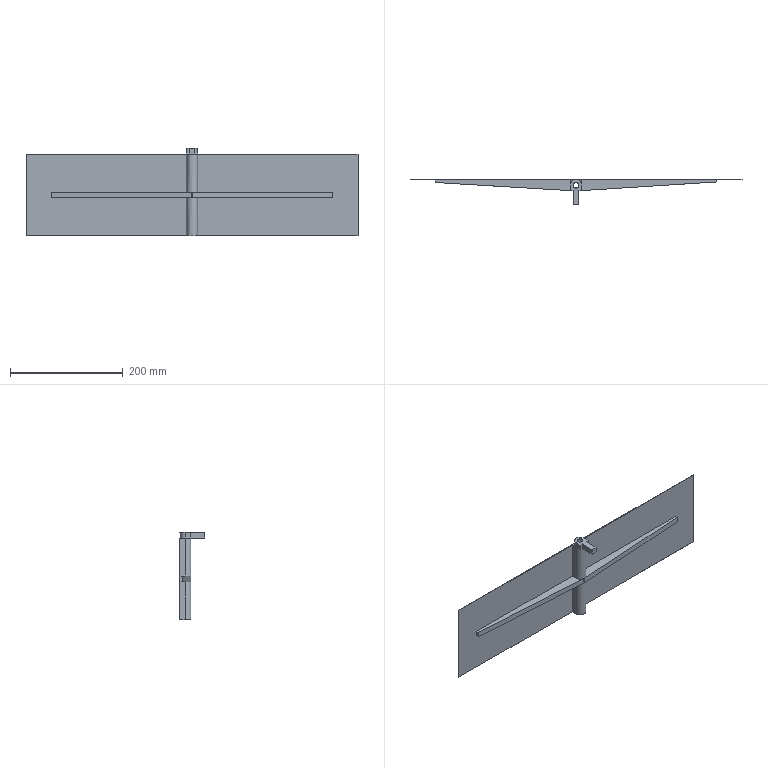Part | SolidWorks | features ICE 3, Extrusion 1 | 1 solid | 32 faces | box 590 x 46 x 155 mm | volume 188951 mm3 | plane 28 | cylinder 4 | commonest cylinder face diameters 10 x2 20 x2
STEP:
#1=CARTESIAN_POINT('',(-5.,0.,82.5));
#2=VERTEX_POINT('',#1);
#3=CARTESIAN_POINT('',(5.,0.,82.5));
#4=VERTEX_POINT('',#3);
#5=CARTESIAN_POINT('',(0.,0.,82.5));
#6=DIRECTION('',(0.,0.,1.));
#7=DIRECTION('',(1.,0.,0.));
#8=AXIS2_PLACEMENT_3D('',#5,#6,#7);
#9=CIRCLE('',#8,5.);
#10=EDGE_CURVE('',#2,#4,#9,.T.);
#11=ORIENTED_EDGE('',*,*,#10,.T.);
#12=CARTESIAN_POINT('',(5.,0.,-72.5));
#13=VERTEX_POINT('',#12);
#14=CARTESIAN_POINT('',(5.,0.,72.5));
#15=DIRECTION('',(0.,0.,-1.));
#16=VECTOR('',#15,1000.);
#17=LINE('',#14,#16);
#18=EDGE_CURVE('',#4,#13,#17,.T.);
#19=ORIENTED_EDGE('',*,*,#18,.T.);
#20=CARTESIAN_POINT('',(-5.,0.,-72.5));
#21=VERTEX_POINT('',#20);
#22=CARTESIAN_POINT('',(0.,0.,-72.5));
#23=DIRECTION('',(0.,0.,1.));
#24=DIRECTION('',(1.,0.,0.));
#25=AXIS2_PLACEMENT_3D('',#22,#23,#24);
#26=CIRCLE('',#25,5.);
#27=EDGE_CURVE('',#21,#13,#26,.T.);
#28=ORIENTED_EDGE('',*,*,#27,.F.);
#29=CARTESIAN_POINT('',(-5.,0.,72.5));
#30=DIRECTION('',(0.,0.,-1.));
#31=VECTOR('',#30,1000.);
#32=LINE('',#29,#31);
#33=EDGE_CURVE('',#2,#21,#32,.T.);
#34=ORIENTED_EDGE('',*,*,#33,.F.);
#35=EDGE_LOOP('',(#11,#19,#28,#34));
#36=FACE_OUTER_BOUND('',#35,.T.);
#37=CARTESIAN_POINT('',(0.,0.,72.5));
#38=DIRECTION('',(0.,0.,-1.));
#39=DIRECTION('',(-1.,0.,0.));
#40=AXIS2_PLACEMENT_3D('',#37,#38,#39);
#41=CYLINDRICAL_SURFACE('',#40,5.);
#42=ADVANCED_FACE('',(#36),#41,.F.);
#43=CARTESIAN_POINT('',(10.,10.,-5.));
#44=VERTEX_POINT('',#43);
#45=CARTESIAN_POINT('',(10.,0.,-5.));
#46=VERTEX_POINT('',#45);
#47=CARTESIAN_POINT('',(10.,0.,-5.));
#48=DIRECTION('',(0.,-1.,0.));
#49=VECTOR('',#48,1000.);
#50=LINE('',#47,#49);
#51=EDGE_CURVE('',#44,#46,#50,.T.);
#52=ORIENTED_EDGE('',*,*,#51,.T.);
#53=CARTESIAN_POINT('',(10.,0.,-72.5));
#54=VERTEX_POINT('',#53);
#55=CARTESIAN_POINT('',(10.,0.,72.5));
#56=DIRECTION('',(0.,0.,-1.));
#57=VECTOR('',#56,1000.);
#58=LINE('',#55,#57);
#59=EDGE_CURVE('',#46,#54,#58,.T.);
#60=ORIENTED_EDGE('',*,*,#59,.T.);
#61=CARTESIAN_POINT('',(10.,10.,-72.5));
#62=VERTEX_POINT('',#61);
#63=CARTESIAN_POINT('',(10.,10.,-72.5));
#64=DIRECTION('',(0.,1.,0.));
#65=VECTOR('',#64,1000.);
#66=LINE('',#63,#65);
#67=EDGE_CURVE('',#54,#62,#66,.T.);
#68=ORIENTED_EDGE('',*,*,#67,.T.);
#69=CARTESIAN_POINT('',(10.,10.,72.5));
#70=DIRECTION('',(0.,0.,-1.));
#71=VECTOR('',#70,1000.);
#72=LINE('',#69,#71);
#73=EDGE_CURVE('',#44,#62,#72,.T.);
#74=ORIENTED_EDGE('',*,*,#73,.F.);
#75=EDGE_LOOP('',(#52,#60,#68,#74));
#76=FACE_OUTER_BOUND('',#75,.T.);
#77=CARTESIAN_POINT('',(10.,10.,72.5));
#78=DIRECTION('',(-1.,0.,0.));
#79=DIRECTION('',(0.,0.,1.));
#80=AXIS2_PLACEMENT_3D('',#77,#78,#79);
#81=PLANE('',#80);
#82=ADVANCED_FACE('',(#76),#81,.F.);
#83=CARTESIAN_POINT('',(-10.,0.,-5.));
#84=VERTEX_POINT('',#83);
#85=CARTESIAN_POINT('',(-10.,10.,-5.));
#86=VERTEX_POINT('',#85);
#87=CARTESIAN_POINT('',(-10.,10.,-5.));
#88=DIRECTION('',(0.,1.,0.));
#89=VECTOR('',#88,1000.);
#90=LINE('',#87,#89);
#91=EDGE_CURVE('',#84,#86,#90,.T.);
#92=ORIENTED_EDGE('',*,*,#91,.T.);
#93=CARTESIAN_POINT('',(-10.,10.,-72.5));
#94=VERTEX_POINT('',#93);
#95=CARTESIAN_POINT('',(-10.,10.,72.5));
#96=DIRECTION('',(0.,0.,-1.));
#97=VECTOR('',#96,1000.);
#98=LINE('',#95,#97);
#99=EDGE_CURVE('',#86,#94,#98,.T.);
#100=ORIENTED_EDGE('',*,*,#99,.T.);
#101=CARTESIAN_POINT('',(-10.,0.,-72.5));
#102=VERTEX_POINT('',#101);
#103=CARTESIAN_POINT('',(-10.,0.,-72.5));
#104=DIRECTION('',(0.,-1.,0.));
#105=VECTOR('',#104,1000.);
#106=LINE('',#103,#105);
#107=EDGE_CURVE('',#94,#102,#106,.T.);
#108=ORIENTED_EDGE('',*,*,#107,.T.);
#109=CARTESIAN_POINT('',(-10.,0.,72.5));
#110=DIRECTION('',(0.,0.,-1.));
#111=VECTOR('',#110,1000.);
#112=LINE('',#109,#111);
#113=EDGE_CURVE('',#84,#102,#112,.T.);
#114=ORIENTED_EDGE('',*,*,#113,.F.);
#115=EDGE_LOOP('',(#92,#100,#108,#114));
#116=FACE_OUTER_BOUND('',#115,.T.);
#117=CARTESIAN_POINT('',(-10.,0.,72.5));
#118=DIRECTION('',(1.,0.,0.));
#119=DIRECTION('',(0.,0.,-1.));
#120=AXIS2_PLACEMENT_3D('',#117,#118,#119);
#121=PLANE('',#120);
#122=ADVANCED_FACE('',(#116),#121,.F.);
#123=CARTESIAN_POINT('',(10.,0.,72.5));
#124=VERTEX_POINT('',#123);
#125=CARTESIAN_POINT('',(-10.,0.,72.5));
#126=VERTEX_POINT('',#125);
#127=CARTESIAN_POINT('',(0.,0.,72.5));
#128=DIRECTION('',(0.,0.,1.));
#129=DIRECTION('',(1.,0.,0.));
#130=AXIS2_PLACEMENT_3D('',#127,#128,#129);
#131=CIRCLE('',#130,10.);
#132=EDGE_CURVE('',#124,#126,#131,.T.);
#133=ORIENTED_EDGE('',*,*,#132,.F.);
#134=CARTESIAN_POINT('',(10.,10.,72.5));
#135=VERTEX_POINT('',#134);
#136=CARTESIAN_POINT('',(10.,10.,72.5));
#137=DIRECTION('',(0.,1.,0.));
#138=VECTOR('',#137,1000.);
#139=LINE('',#136,#138);
#140=EDGE_CURVE('',#124,#135,#139,.T.);
#141=ORIENTED_EDGE('',*,*,#140,.T.);
#142=CARTESIAN_POINT('',(295.,10.,72.5));
#143=VERTEX_POINT('',#142);
#144=CARTESIAN_POINT('',(-295.,10.,72.5));
#145=DIRECTION('',(1.,0.,0.));
#146=VECTOR('',#145,1000.);
#147=LINE('',#144,#146);
#148=EDGE_CURVE('',#135,#143,#147,.T.);
#149=ORIENTED_EDGE('',*,*,#148,.T.);
#150=CARTESIAN_POINT('',(295.,11.,72.5));
#151=VERTEX_POINT('',#150);
#152=CARTESIAN_POINT('',(295.,11.,72.5));
#153=DIRECTION('',(0.,-1.,0.));
#154=VECTOR('',#153,1000.);
#155=LINE('',#152,#154);
#156=EDGE_CURVE('',#151,#143,#155,.T.);
#157=ORIENTED_EDGE('',*,*,#156,.F.);
#158=CARTESIAN_POINT('',(-295.,11.,72.5));
#159=VERTEX_POINT('',#158);
#160=CARTESIAN_POINT('',(-295.,11.,72.5));
#161=DIRECTION('',(1.,0.,0.));
#162=VECTOR('',#161,1000.);
#163=LINE('',#160,#162);
#164=EDGE_CURVE('',#159,#151,#163,.T.);
#165=ORIENTED_EDGE('',*,*,#164,.F.);
#166=CARTESIAN_POINT('',(-295.,10.,72.5));
#167=VERTEX_POINT('',#166);
#168=CARTESIAN_POINT('',(-295.,11.,72.5));
#169=DIRECTION('',(0.,-1.,0.));
#170=VECTOR('',#169,1000.);
#171=LINE('',#168,#170);
#172=EDGE_CURVE('',#159,#167,#171,.T.);
#173=ORIENTED_EDGE('',*,*,#172,.T.);
#174=CARTESIAN_POINT('',(-10.,10.,72.5));
#175=VERTEX_POINT('',#174);
#176=CARTESIAN_POINT('',(-295.,10.,72.5));
#177=DIRECTION('',(1.,0.,0.));
#178=VECTOR('',#177,1000.);
#179=LINE('',#176,#178);
#180=EDGE_CURVE('',#167,#175,#179,.T.);
#181=ORIENTED_EDGE('',*,*,#180,.T.);
#182=CARTESIAN_POINT('',(-10.,0.,72.5));
#183=DIRECTION('',(0.,-1.,0.));
#184=VECTOR('',#183,1000.);
#185=LINE('',#182,#184);
#186=EDGE_CURVE('',#175,#126,#185,.T.);
#187=ORIENTED_EDGE('',*,*,#186,.T.);
#188=EDGE_LOOP('',(#133,#141,#149,#157,#165,#173,#181,#187));
#189=FACE_OUTER_BOUND('',#188,.T.);
#190=CARTESIAN_POINT('',(0.,0.,72.5));
#191=DIRECTION('',(0.,0.,1.));
#192=DIRECTION('',(1.,0.,0.));
#193=AXIS2_PLACEMENT_3D('',#190,#191,#192);
#194=PLANE('',#193);
#195=ADVANCED_FACE('',(#189),#194,.T.);
#196=CARTESIAN_POINT('',(0.,0.,-72.5));
#197=DIRECTION('',(0.,0.,1.));
#198=DIRECTION('',(1.,0.,0.));
#199=AXIS2_PLACEMENT_3D('',#196,#197,#198);
#200=CIRCLE('',#199,10.);
#201=EDGE_CURVE('',#102,#54,#200,.T.);
#202=ORIENTED_EDGE('',*,*,#201,.F.);
#203=ORIENTED_EDGE('',*,*,#107,.F.);
#204=CARTESIAN_POINT('',(-295.,10.,-72.5));
#205=VERTEX_POINT('',#204);
#206=CARTESIAN_POINT('',(-295.,10.,-72.5));
#207=DIRECTION('',(-1.,0.,0.));
#208=VECTOR('',#207,1000.);
#209=LINE('',#206,#208);
#210=EDGE_CURVE('',#94,#205,#209,.T.);
#211=ORIENTED_EDGE('',*,*,#210,.T.);
#212=CARTESIAN_POINT('',(-295.,11.,-72.5));
#213=VERTEX_POINT('',#212);
#214=CARTESIAN_POINT('',(-295.,11.,-72.5));
#215=DIRECTION('',(0.,-1.,0.));
#216=VECTOR('',#215,1000.);
#217=LINE('',#214,#216);
#218=EDGE_CURVE('',#213,#205,#217,.T.);
#219=ORIENTED_EDGE('',*,*,#218,.F.);
#220=CARTESIAN_POINT('',(295.,11.,-72.5));
#221=VERTEX_POINT('',#220);
#222=CARTESIAN_POINT('',(-295.,11.,-72.5));
#223=DIRECTION('',(-1.,0.,0.));
#224=VECTOR('',#223,1000.);
#225=LINE('',#222,#224);
#226=EDGE_CURVE('',#221,#213,#225,.T.);
#227=ORIENTED_EDGE('',*,*,#226,.F.);
#228=CARTESIAN_POINT('',(295.,10.,-72.5));
#229=VERTEX_POINT('',#228);
#230=CARTESIAN_POINT('',(295.,11.,-72.5));
#231=DIRECTION('',(0.,-1.,0.));
#232=VECTOR('',#231,1000.);
#233=LINE('',#230,#232);
#234=EDGE_CURVE('',#221,#229,#233,.T.);
#235=ORIENTED_EDGE('',*,*,#234,.T.);
#236=CARTESIAN_POINT('',(-295.,10.,-72.5));
#237=DIRECTION('',(-1.,0.,0.));
#238=VECTOR('',#237,1000.);
#239=LINE('',#236,#238);
#240=EDGE_CURVE('',#229,#62,#239,.T.);
#241=ORIENTED_EDGE('',*,*,#240,.T.);
#242=ORIENTED_EDGE('',*,*,#67,.F.);
#243=EDGE_LOOP('',(#202,#203,#211,#219,#227,#235,#241,#242));
#244=FACE_OUTER_BOUND('',#243,.T.);
#245=ORIENTED_EDGE('',*,*,#27,.T.);
#246=CARTESIAN_POINT('',(0.,0.,-72.5));
#247=DIRECTION('',(0.,0.,1.));
#248=DIRECTION('',(1.,0.,0.));
#249=AXIS2_PLACEMENT_3D('',#246,#247,#248);
#250=CIRCLE('',#249,5.);
#251=EDGE_CURVE('',#13,#21,#250,.T.);
#252=ORIENTED_EDGE('',*,*,#251,.T.);
#253=EDGE_LOOP('',(#245,#252));
#254=FACE_BOUND('',#253,.T.);
#255=CARTESIAN_POINT('',(0.,0.,-72.5));
#256=DIRECTION('',(0.,0.,1.));
#257=DIRECTION('',(1.,0.,0.));
#258=AXIS2_PLACEMENT_3D('',#255,#256,#257);
#259=PLANE('',#258);
#260=ADVANCED_FACE('',(#244,#254),#259,.F.);
#261=CARTESIAN_POINT('',(0.6395,-9.98,5.));
#262=VERTEX_POINT('',#261);
#263=CARTESIAN_POINT('',(0.6395,-9.98,-5.));
#264=VERTEX_POINT('',#263);
#265=CARTESIAN_POINT('',(0.6395,-9.98,5.));
#266=DIRECTION('',(0.,0.,-1.));
#267=VECTOR('',#266,1000.);
#268=LINE('',#265,#267);
#269=EDGE_CURVE('',#262,#264,#268,.T.);
#270=ORIENTED_EDGE('',*,*,#269,.F.);
#271=CARTESIAN_POINT('',(10.,0.,5.));
#272=VERTEX_POINT('',#271);
#273=CARTESIAN_POINT('',(0.,0.,5.));
#274=DIRECTION('',(0.,0.,-1.));
#275=DIRECTION('',(1.,0.,0.));
#276=AXIS2_PLACEMENT_3D('',#273,#274,#275);
#277=CIRCLE('',#276,10.);
#278=EDGE_CURVE('',#272,#262,#277,.T.);
#279=ORIENTED_EDGE('',*,*,#278,.F.);
#280=CARTESIAN_POINT('',(10.,0.,72.5));
#281=DIRECTION('',(0.,0.,-1.));
#282=VECTOR('',#281,1000.);
#283=LINE('',#280,#282);
#284=EDGE_CURVE('',#124,#272,#283,.T.);
#285=ORIENTED_EDGE('',*,*,#284,.F.);
#286=CARTESIAN_POINT('',(0.,0.,72.5));
#287=DIRECTION('',(0.,0.,1.));
#288=DIRECTION('',(1.,0.,0.));
#289=AXIS2_PLACEMENT_3D('',#286,#287,#288);
#290=CIRCLE('',#289,10.);
#291=EDGE_CURVE('',#126,#124,#290,.T.);
#292=ORIENTED_EDGE('',*,*,#291,.F.);
#293=CARTESIAN_POINT('',(-10.,0.,5.));
#294=VERTEX_POINT('',#293);
#295=CARTESIAN_POINT('',(-10.,0.,72.5));
#296=DIRECTION('',(0.,0.,-1.));
#297=VECTOR('',#296,1000.);
#298=LINE('',#295,#297);
#299=EDGE_CURVE('',#126,#294,#298,.T.);
#300=ORIENTED_EDGE('',*,*,#299,.T.);
#301=CARTESIAN_POINT('',(-0.5996,-9.982,5.));
#302=VERTEX_POINT('',#301);
#303=CARTESIAN_POINT('',(0.,0.,5.));
#304=DIRECTION('',(0.,0.,-1.));
#305=DIRECTION('',(1.,0.,0.));
#306=AXIS2_PLACEMENT_3D('',#303,#304,#305);
#307=CIRCLE('',#306,10.);
#308=EDGE_CURVE('',#302,#294,#307,.T.);
#309=ORIENTED_EDGE('',*,*,#308,.F.);
#310=CARTESIAN_POINT('',(-0.5996,-9.982,-5.));
#311=VERTEX_POINT('',#310);
#312=CARTESIAN_POINT('',(-0.5996,-9.982,5.));
#313=DIRECTION('',(0.,0.,-1.));
#314=VECTOR('',#313,1000.);
#315=LINE('',#312,#314);
#316=EDGE_CURVE('',#302,#311,#315,.T.);
#317=ORIENTED_EDGE('',*,*,#316,.T.);
#318=CARTESIAN_POINT('',(0.,0.,-5.));
#319=DIRECTION('',(0.,0.,-1.));
#320=DIRECTION('',(1.,0.,0.));
#321=AXIS2_PLACEMENT_3D('',#318,#319,#320);
#322=CIRCLE('',#321,10.);
#323=EDGE_CURVE('',#311,#84,#322,.T.);
#324=ORIENTED_EDGE('',*,*,#323,.T.);
#325=ORIENTED_EDGE('',*,*,#113,.T.);
#326=ORIENTED_EDGE('',*,*,#201,.T.);
#327=ORIENTED_EDGE('',*,*,#59,.F.);
#328=CARTESIAN_POINT('',(0.,0.,-5.));
#329=DIRECTION('',(0.,0.,-1.));
#330=DIRECTION('',(1.,0.,0.));
#331=AXIS2_PLACEMENT_3D('',#328,#329,#330);
#332=CIRCLE('',#331,10.);
#333=EDGE_CURVE('',#46,#264,#332,.T.);
#334=ORIENTED_EDGE('',*,*,#333,.T.);
#335=EDGE_LOOP('',(#270,#279,#285,#292,#300,#309,#317,#324,#325,#326,#327,#334));
#336=FACE_OUTER_BOUND('',#335,.T.);
#337=CARTESIAN_POINT('',(0.,0.,72.5));
#338=DIRECTION('',(0.,0.,-1.));
#339=DIRECTION('',(-1.,0.,0.));
#340=AXIS2_PLACEMENT_3D('',#337,#338,#339);
#341=CYLINDRICAL_SURFACE('',#340,10.);
#342=ADVANCED_FACE('',(#336),#341,.T.);
#343=ORIENTED_EDGE('',*,*,#284,.T.);
#344=CARTESIAN_POINT('',(10.,10.,5.));
#345=VERTEX_POINT('',#344);
#346=CARTESIAN_POINT('',(10.,0.,5.));
#347=DIRECTION('',(0.,-1.,0.));
#348=VECTOR('',#347,1000.);
#349=LINE('',#346,#348);
#350=EDGE_CURVE('',#345,#272,#349,.T.);
#351=ORIENTED_EDGE('',*,*,#350,.F.);
#352=CARTESIAN_POINT('',(10.,10.,72.5));
#353=DIRECTION('',(0.,0.,-1.));
#354=VECTOR('',#353,1000.);
#355=LINE('',#352,#354);
#356=EDGE_CURVE('',#135,#345,#355,.T.);
#357=ORIENTED_EDGE('',*,*,#356,.F.);
#358=ORIENTED_EDGE('',*,*,#140,.F.);
#359=EDGE_LOOP('',(#343,#351,#357,#358));
#360=FACE_OUTER_BOUND('',#359,.T.);
#361=CARTESIAN_POINT('',(10.,10.,72.5));
#362=DIRECTION('',(-1.,0.,0.));
#363=DIRECTION('',(0.,0.,1.));
#364=AXIS2_PLACEMENT_3D('',#361,#362,#363);
#365=PLANE('',#364);
#366=ADVANCED_FACE('',(#360),#365,.F.);
#367=CARTESIAN_POINT('',(-10.,10.,5.));
#368=VERTEX_POINT('',#367);
#369=CARTESIAN_POINT('',(-10.,10.,72.5));
#370=DIRECTION('',(0.,0.,-1.));
#371=VECTOR('',#370,1000.);
#372=LINE('',#369,#371);
#373=EDGE_CURVE('',#175,#368,#372,.T.);
#374=ORIENTED_EDGE('',*,*,#373,.T.);
#375=CARTESIAN_POINT('',(-10.,10.,5.));
#376=DIRECTION('',(0.,1.,0.));
#377=VECTOR('',#376,1000.);
#378=LINE('',#375,#377);
#379=EDGE_CURVE('',#294,#368,#378,.T.);
#380=ORIENTED_EDGE('',*,*,#379,.F.);
#381=ORIENTED_EDGE('',*,*,#299,.F.);
#382=ORIENTED_EDGE('',*,*,#186,.F.);
#383=EDGE_LOOP('',(#374,#380,#381,#382));
#384=FACE_OUTER_BOUND('',#383,.T.);
#385=CARTESIAN_POINT('',(-10.,0.,72.5));
#386=DIRECTION('',(1.,0.,0.));
#387=DIRECTION('',(0.,0.,-1.));
#388=AXIS2_PLACEMENT_3D('',#385,#386,#387);
#389=PLANE('',#388);
#390=ADVANCED_FACE('',(#384),#389,.F.);
#391=ORIENTED_EDGE('',*,*,#18,.F.);
#392=CARTESIAN_POINT('',(0.,0.,82.5));
#393=DIRECTION('',(0.,0.,1.));
#394=DIRECTION('',(1.,0.,0.));
#395=AXIS2_PLACEMENT_3D('',#392,#393,#394);
#396=CIRCLE('',#395,5.);
#397=EDGE_CURVE('',#4,#2,#396,.T.);
#398=ORIENTED_EDGE('',*,*,#397,.T.);
#399=ORIENTED_EDGE('',*,*,#33,.T.);
#400=ORIENTED_EDGE('',*,*,#251,.F.);
#401=EDGE_LOOP('',(#391,#398,#399,#400));
#402=FACE_OUTER_BOUND('',#401,.T.);
#403=CARTESIAN_POINT('',(0.,0.,72.5));
#404=DIRECTION('',(0.,0.,-1.));
#405=DIRECTION('',(-1.,0.,0.));
#406=AXIS2_PLACEMENT_3D('',#403,#404,#405);
#407=CYLINDRICAL_SURFACE('',#406,5.);
#408=ADVANCED_FACE('',(#402),#407,.F.);
#409=CARTESIAN_POINT('',(-250.,10.,-5.));
#410=VERTEX_POINT('',#409);
#411=CARTESIAN_POINT('',(-250.,5.,-5.));
#412=VERTEX_POINT('',#411);
#413=CARTESIAN_POINT('',(-250.,10.,-5.));
#414=DIRECTION('',(0.,-1.,0.));
#415=VECTOR('',#414,1000.);
#416=LINE('',#413,#415);
#417=EDGE_CURVE('',#410,#412,#416,.T.);
#418=ORIENTED_EDGE('',*,*,#417,.T.);
#419=CARTESIAN_POINT('',(-250.,5.,5.));
#420=VERTEX_POINT('',#419);
#421=CARTESIAN_POINT('',(-250.,5.,5.));
#422=DIRECTION('',(0.,0.,-1.));
#423=VECTOR('',#422,1000.);
#424=LINE('',#421,#423);
#425=EDGE_CURVE('',#420,#412,#424,.T.);
#426=ORIENTED_EDGE('',*,*,#425,.F.);
#427=CARTESIAN_POINT('',(-250.,10.,5.));
#428=VERTEX_POINT('',#427);
#429=CARTESIAN_POINT('',(-250.,10.,5.));
#430=DIRECTION('',(0.,-1.,0.));
#431=VECTOR('',#430,1000.);
#432=LINE('',#429,#431);
#433=EDGE_CURVE('',#428,#420,#432,.T.);
#434=ORIENTED_EDGE('',*,*,#433,.F.);
#435=CARTESIAN_POINT('',(-250.,10.,5.));
#436=DIRECTION('',(0.,0.,-1.));
#437=VECTOR('',#436,1000.);
#438=LINE('',#435,#437);
#439=EDGE_CURVE('',#428,#410,#438,.T.);
#440=ORIENTED_EDGE('',*,*,#439,.T.);
#441=EDGE_LOOP('',(#418,#426,#434,#440));
#442=FACE_OUTER_BOUND('',#441,.T.);
#443=CARTESIAN_POINT('',(-250.,10.,5.));
#444=DIRECTION('',(1.,0.,0.));
#445=DIRECTION('',(0.,0.,-1.));
#446=AXIS2_PLACEMENT_3D('',#443,#444,#445);
#447=PLANE('',#446);
#448=ADVANCED_FACE('',(#442),#447,.F.);
#449=CARTESIAN_POINT('',(-250.,5.,-5.));
#450=DIRECTION('',(0.9982,-0.05996,0.));
#451=VECTOR('',#450,1000.);
#452=LINE('',#449,#451);
#453=EDGE_CURVE('',#412,#311,#452,.T.);
#454=ORIENTED_EDGE('',*,*,#453,.T.);
#455=ORIENTED_EDGE('',*,*,#316,.F.);
#456=CARTESIAN_POINT('',(-250.,5.,5.));
#457=DIRECTION('',(0.9982,-0.05996,0.));
#458=VECTOR('',#457,1000.);
#459=LINE('',#456,#458);
#460=EDGE_CURVE('',#420,#302,#459,.T.);
#461=ORIENTED_EDGE('',*,*,#460,.F.);
#462=ORIENTED_EDGE('',*,*,#425,.T.);
#463=EDGE_LOOP('',(#454,#455,#461,#462));
#464=FACE_OUTER_BOUND('',#463,.T.);
#465=CARTESIAN_POINT('',(-250.,5.,5.));
#466=DIRECTION('',(0.05996,0.9982,0.));
#467=DIRECTION('',(-0.9982,0.05996,0.));
#468=AXIS2_PLACEMENT_3D('',#465,#466,#467);
#469=PLANE('',#468);
#470=ADVANCED_FACE('',(#464),#469,.F.);
#471=ORIENTED_EDGE('',*,*,#379,.T.);
#472=CARTESIAN_POINT('',(-10.,10.,5.));
#473=DIRECTION('',(-1.,0.,0.));
#474=VECTOR('',#473,1000.);
#475=LINE('',#472,#474);
#476=EDGE_CURVE('',#368,#428,#475,.T.);
#477=ORIENTED_EDGE('',*,*,#476,.T.);
#478=ORIENTED_EDGE('',*,*,#433,.T.);
#479=ORIENTED_EDGE('',*,*,#460,.T.);
#480=ORIENTED_EDGE('',*,*,#308,.T.);
#481=EDGE_LOOP('',(#471,#477,#478,#479,#480));
#482=FACE_OUTER_BOUND('',#481,.T.);
#483=CARTESIAN_POINT('',(0.,0.,5.));
#484=DIRECTION('',(0.,0.,1.));
#485=DIRECTION('',(1.,0.,0.));
#486=AXIS2_PLACEMENT_3D('',#483,#484,#485);
#487=PLANE('',#486);
#488=ADVANCED_FACE('',(#482),#487,.T.);
#489=ORIENTED_EDGE('',*,*,#91,.F.);
#490=ORIENTED_EDGE('',*,*,#323,.F.);
#491=ORIENTED_EDGE('',*,*,#453,.F.);
#492=ORIENTED_EDGE('',*,*,#417,.F.);
#493=CARTESIAN_POINT('',(-10.,10.,-5.));
#494=DIRECTION('',(-1.,0.,0.));
#495=VECTOR('',#494,1000.);
#496=LINE('',#493,#495);
#497=EDGE_CURVE('',#86,#410,#496,.T.);
#498=ORIENTED_EDGE('',*,*,#497,.F.);
#499=EDGE_LOOP('',(#489,#490,#491,#492,#498));
#500=FACE_OUTER_BOUND('',#499,.T.);
#501=CARTESIAN_POINT('',(0.,0.,-5.));
#502=DIRECTION('',(0.,0.,1.));
#503=DIRECTION('',(1.,0.,0.));
#504=AXIS2_PLACEMENT_3D('',#501,#502,#503);
#505=PLANE('',#504);
#506=ADVANCED_FACE('',(#500),#505,.F.);
#507=ORIENTED_EDGE('',*,*,#356,.T.);
#508=CARTESIAN_POINT('',(249.998,10.,5.));
#509=VERTEX_POINT('',#508);
#510=CARTESIAN_POINT('',(0.,10.,5.));
#511=DIRECTION('',(1.,0.,0.));
#512=VECTOR('',#511,1000.);
#513=LINE('',#510,#512);
#514=EDGE_CURVE('',#345,#509,#513,.T.);
#515=ORIENTED_EDGE('',*,*,#514,.T.);
#516=CARTESIAN_POINT('',(249.998,10.,-5.));
#517=VERTEX_POINT('',#516);
#518=CARTESIAN_POINT('',(249.998,10.,0.));
#519=DIRECTION('',(0.,0.,1.));
#520=VECTOR('',#519,1000.);
#521=LINE('',#518,#520);
#522=EDGE_CURVE('',#517,#509,#521,.T.);
#523=ORIENTED_EDGE('',*,*,#522,.F.);
#524=CARTESIAN_POINT('',(0.,10.,-5.));
#525=DIRECTION('',(1.,0.,0.));
#526=VECTOR('',#525,1000.);
#527=LINE('',#524,#526);
#528=EDGE_CURVE('',#44,#517,#527,.T.);
#529=ORIENTED_EDGE('',*,*,#528,.F.);
#530=ORIENTED_EDGE('',*,*,#73,.T.);
#531=ORIENTED_EDGE('',*,*,#240,.F.);
#532=CARTESIAN_POINT('',(295.,10.,-72.5));
#533=DIRECTION('',(0.,0.,-1.));
#534=VECTOR('',#533,1000.);
#535=LINE('',#532,#534);
#536=EDGE_CURVE('',#143,#229,#535,.T.);
#537=ORIENTED_EDGE('',*,*,#536,.F.);
#538=ORIENTED_EDGE('',*,*,#148,.F.);
#539=EDGE_LOOP('',(#507,#515,#523,#529,#530,#531,#537,#538));
#540=FACE_OUTER_BOUND('',#539,.T.);
#541=CARTESIAN_POINT('',(0.,10.,0.));
#542=DIRECTION('',(0.,1.,0.));
#543=DIRECTION('',(0.,0.,1.));
#544=AXIS2_PLACEMENT_3D('',#541,#542,#543);
#545=PLANE('',#544);
#546=ADVANCED_FACE('',(#540),#545,.F.);
#547=CARTESIAN_POINT('',(-295.,10.,-72.5));
#548=DIRECTION('',(0.,0.,1.));
#549=VECTOR('',#548,1000.);
#550=LINE('',#547,#549);
#551=EDGE_CURVE('',#205,#167,#550,.T.);
#552=ORIENTED_EDGE('',*,*,#551,.T.);
#553=ORIENTED_EDGE('',*,*,#172,.F.);
#554=CARTESIAN_POINT('',(-295.,11.,-72.5));
#555=DIRECTION('',(0.,0.,1.));
#556=VECTOR('',#555,1000.);
#557=LINE('',#554,#556);
#558=EDGE_CURVE('',#213,#159,#557,.T.);
#559=ORIENTED_EDGE('',*,*,#558,.F.);
#560=ORIENTED_EDGE('',*,*,#218,.T.);
#561=EDGE_LOOP('',(#552,#553,#559,#560));
#562=FACE_OUTER_BOUND('',#561,.T.);
#563=CARTESIAN_POINT('',(-295.,11.,-72.5));
#564=DIRECTION('',(1.,0.,0.));
#565=DIRECTION('',(0.,0.,-1.));
#566=AXIS2_PLACEMENT_3D('',#563,#564,#565);
#567=PLANE('',#566);
#568=ADVANCED_FACE('',(#562),#567,.F.);
#569=ORIENTED_EDGE('',*,*,#536,.T.);
#570=ORIENTED_EDGE('',*,*,#234,.F.);
#571=CARTESIAN_POINT('',(295.,11.,-72.5));
#572=DIRECTION('',(0.,0.,-1.));
#573=VECTOR('',#572,1000.);
#574=LINE('',#571,#573);
#575=EDGE_CURVE('',#151,#221,#574,.T.);
#576=ORIENTED_EDGE('',*,*,#575,.F.);
#577=ORIENTED_EDGE('',*,*,#156,.T.);
#578=EDGE_LOOP('',(#569,#570,#576,#577));
#579=FACE_OUTER_BOUND('',#578,.T.);
#580=CARTESIAN_POINT('',(295.,11.,-72.5));
#581=DIRECTION('',(-1.,0.,0.));
#582=DIRECTION('',(0.,0.,1.));
#583=AXIS2_PLACEMENT_3D('',#580,#581,#582);
#584=PLANE('',#583);
#585=ADVANCED_FACE('',(#579),#584,.F.);
#586=ORIENTED_EDGE('',*,*,#558,.T.);
#587=ORIENTED_EDGE('',*,*,#164,.T.);
#588=ORIENTED_EDGE('',*,*,#575,.T.);
#589=ORIENTED_EDGE('',*,*,#226,.T.);
#590=EDGE_LOOP('',(#586,#587,#588,#589));
#591=FACE_OUTER_BOUND('',#590,.T.);
#592=CARTESIAN_POINT('',(0.,11.,0.));
#593=DIRECTION('',(0.,1.,0.));
#594=DIRECTION('',(0.,0.,1.));
#595=AXIS2_PLACEMENT_3D('',#592,#593,#594);
#596=PLANE('',#595);
#597=ADVANCED_FACE('',(#591),#596,.T.);
#598=ORIENTED_EDGE('',*,*,#99,.F.);
#599=ORIENTED_EDGE('',*,*,#497,.T.);
#600=ORIENTED_EDGE('',*,*,#439,.F.);
#601=ORIENTED_EDGE('',*,*,#476,.F.);
#602=ORIENTED_EDGE('',*,*,#373,.F.);
#603=ORIENTED_EDGE('',*,*,#180,.F.);
#604=ORIENTED_EDGE('',*,*,#551,.F.);
#605=ORIENTED_EDGE('',*,*,#210,.F.);
#606=EDGE_LOOP('',(#598,#599,#600,#601,#602,#603,#604,#605));
#607=FACE_OUTER_BOUND('',#606,.T.);
#608=CARTESIAN_POINT('',(0.,10.,0.));
#609=DIRECTION('',(0.,1.,0.));
#610=DIRECTION('',(0.,0.,1.));
#611=AXIS2_PLACEMENT_3D('',#608,#609,#610);
#612=PLANE('',#611);
#613=ADVANCED_FACE('',(#607),#612,.F.);
#614=CARTESIAN_POINT('',(249.998,6.,-5.));
#615=VERTEX_POINT('',#614);
#616=CARTESIAN_POINT('',(249.998,11.,-5.));
#617=DIRECTION('',(0.,1.,0.));
#618=VECTOR('',#617,1000.);
#619=LINE('',#616,#618);
#620=EDGE_CURVE('',#615,#517,#619,.T.);
#621=ORIENTED_EDGE('',*,*,#620,.T.);
#622=ORIENTED_EDGE('',*,*,#522,.T.);
#623=CARTESIAN_POINT('',(249.998,6.,5.));
#624=VERTEX_POINT('',#623);
#625=CARTESIAN_POINT('',(249.998,11.,5.));
#626=DIRECTION('',(0.,1.,0.));
#627=VECTOR('',#626,1000.);
#628=LINE('',#625,#627);
#629=EDGE_CURVE('',#624,#509,#628,.T.);
#630=ORIENTED_EDGE('',*,*,#629,.F.);
#631=CARTESIAN_POINT('',(249.998,6.,5.));
#632=DIRECTION('',(0.,0.,-1.));
#633=VECTOR('',#632,1000.);
#634=LINE('',#631,#633);
#635=EDGE_CURVE('',#624,#615,#634,.T.);
#636=ORIENTED_EDGE('',*,*,#635,.T.);
#637=EDGE_LOOP('',(#621,#622,#630,#636));
#638=FACE_OUTER_BOUND('',#637,.T.);
#639=CARTESIAN_POINT('',(249.998,11.,5.));
#640=DIRECTION('',(-1.,0.,0.));
#641=DIRECTION('',(0.,0.,1.));
#642=AXIS2_PLACEMENT_3D('',#639,#640,#641);
#643=PLANE('',#642);
#644=ADVANCED_FACE('',(#638),#643,.F.);
#645=ORIENTED_EDGE('',*,*,#514,.F.);
#646=ORIENTED_EDGE('',*,*,#350,.T.);
#647=ORIENTED_EDGE('',*,*,#278,.T.);
#648=CARTESIAN_POINT('',(249.998,6.,5.));
#649=DIRECTION('',(0.998,0.06395,0.));
#650=VECTOR('',#649,1000.);
#651=LINE('',#648,#650);
#652=EDGE_CURVE('',#262,#624,#651,.T.);
#653=ORIENTED_EDGE('',*,*,#652,.T.);
#654=ORIENTED_EDGE('',*,*,#629,.T.);
#655=EDGE_LOOP('',(#645,#646,#647,#653,#654));
#656=FACE_OUTER_BOUND('',#655,.T.);
#657=CARTESIAN_POINT('',(0.,0.,5.));
#658=DIRECTION('',(0.,0.,1.));
#659=DIRECTION('',(1.,0.,0.));
#660=AXIS2_PLACEMENT_3D('',#657,#658,#659);
#661=PLANE('',#660);
#662=ADVANCED_FACE('',(#656),#661,.T.);
#663=ORIENTED_EDGE('',*,*,#51,.F.);
#664=ORIENTED_EDGE('',*,*,#528,.T.);
#665=ORIENTED_EDGE('',*,*,#620,.F.);
#666=CARTESIAN_POINT('',(249.998,6.,-5.));
#667=DIRECTION('',(0.998,0.06395,0.));
#668=VECTOR('',#667,1000.);
#669=LINE('',#666,#668);
#670=EDGE_CURVE('',#264,#615,#669,.T.);
#671=ORIENTED_EDGE('',*,*,#670,.F.);
#672=ORIENTED_EDGE('',*,*,#333,.F.);
#673=EDGE_LOOP('',(#663,#664,#665,#671,#672));
#674=FACE_OUTER_BOUND('',#673,.T.);
#675=CARTESIAN_POINT('',(0.,0.,-5.));
#676=DIRECTION('',(0.,0.,1.));
#677=DIRECTION('',(1.,0.,0.));
#678=AXIS2_PLACEMENT_3D('',#675,#676,#677);
#679=PLANE('',#678);
#680=ADVANCED_FACE('',(#674),#679,.F.);
#681=ORIENTED_EDGE('',*,*,#670,.T.);
#682=ORIENTED_EDGE('',*,*,#635,.F.);
#683=ORIENTED_EDGE('',*,*,#652,.F.);
#684=ORIENTED_EDGE('',*,*,#269,.T.);
#685=EDGE_LOOP('',(#681,#682,#683,#684));
#686=FACE_OUTER_BOUND('',#685,.T.);
#687=CARTESIAN_POINT('',(249.998,6.,5.));
#688=DIRECTION('',(-0.06395,0.998,0.));
#689=DIRECTION('',(-0.998,-0.06395,0.));
#690=AXIS2_PLACEMENT_3D('',#687,#688,#689);
#691=PLANE('',#690);
#692=ADVANCED_FACE('',(#686),#691,.F.);
#693=CARTESIAN_POINT('',(-10.,-10.,72.5));
#694=VERTEX_POINT('',#693);
#695=CARTESIAN_POINT('',(-10.,0.,72.5));
#696=DIRECTION('',(0.,-1.,0.));
#697=VECTOR('',#696,1000.);
#698=LINE('',#695,#697);
#699=EDGE_CURVE('',#126,#694,#698,.T.);
#700=ORIENTED_EDGE('',*,*,#699,.F.);
#701=ORIENTED_EDGE('',*,*,#291,.T.);
#702=CARTESIAN_POINT('',(10.,-10.,72.5));
#703=VERTEX_POINT('',#702);
#704=CARTESIAN_POINT('',(10.,-10.,72.5));
#705=DIRECTION('',(0.,1.,0.));
#706=VECTOR('',#705,1000.);
#707=LINE('',#704,#706);
#708=EDGE_CURVE('',#703,#124,#707,.T.);
#709=ORIENTED_EDGE('',*,*,#708,.F.);
#710=CARTESIAN_POINT('',(5.,-10.,72.5));
#711=VERTEX_POINT('',#710);
#712=CARTESIAN_POINT('',(5.,-10.,72.5));
#713=DIRECTION('',(1.,0.,0.));
#714=VECTOR('',#713,1000.);
#715=LINE('',#712,#714);
#716=EDGE_CURVE('',#711,#703,#715,.T.);
#717=ORIENTED_EDGE('',*,*,#716,.F.);
#718=CARTESIAN_POINT('',(5.,-35.,72.5));
#719=VERTEX_POINT('',#718);
#720=CARTESIAN_POINT('',(5.,-25.,72.5));
#721=DIRECTION('',(0.,1.,0.));
#722=VECTOR('',#721,1000.);
#723=LINE('',#720,#722);
#724=EDGE_CURVE('',#719,#711,#723,.T.);
#725=ORIENTED_EDGE('',*,*,#724,.F.);
#726=CARTESIAN_POINT('',(-5.,-35.,72.5));
#727=VERTEX_POINT('',#726);
#728=CARTESIAN_POINT('',(-5.,-35.,72.5));
#729=DIRECTION('',(1.,0.,0.));
#730=VECTOR('',#729,1000.);
#731=LINE('',#728,#730);
#732=EDGE_CURVE('',#727,#719,#731,.T.);
#733=ORIENTED_EDGE('',*,*,#732,.F.);
#734=CARTESIAN_POINT('',(-5.,-10.,72.5));
#735=VERTEX_POINT('',#734);
#736=CARTESIAN_POINT('',(-5.,-25.,72.5));
#737=DIRECTION('',(0.,-1.,0.));
#738=VECTOR('',#737,1000.);
#739=LINE('',#736,#738);
#740=EDGE_CURVE('',#735,#727,#739,.T.);
#741=ORIENTED_EDGE('',*,*,#740,.F.);
#742=CARTESIAN_POINT('',(-5.,-10.,72.5));
#743=DIRECTION('',(1.,0.,0.));
#744=VECTOR('',#743,1000.);
#745=LINE('',#742,#744);
#746=EDGE_CURVE('',#694,#735,#745,.T.);
#747=ORIENTED_EDGE('',*,*,#746,.F.);
#748=EDGE_LOOP('',(#700,#701,#709,#717,#725,#733,#741,#747));
#749=FACE_OUTER_BOUND('',#748,.T.);
#750=CARTESIAN_POINT('',(0.,0.,72.5));
#751=DIRECTION('',(0.,0.,1.));
#752=DIRECTION('',(1.,0.,0.));
#753=AXIS2_PLACEMENT_3D('',#750,#751,#752);
#754=PLANE('',#753);
#755=ADVANCED_FACE('',(#749),#754,.F.);
#756=CARTESIAN_POINT('',(5.,-35.,82.5));
#757=VERTEX_POINT('',#756);
#758=CARTESIAN_POINT('',(5.,-10.,82.5));
#759=VERTEX_POINT('',#758);
#760=CARTESIAN_POINT('',(5.,-35.,82.5));
#761=DIRECTION('',(0.,1.,0.));
#762=VECTOR('',#761,1000.);
#763=LINE('',#760,#762);
#764=EDGE_CURVE('',#757,#759,#763,.T.);
#765=ORIENTED_EDGE('',*,*,#764,.T.);
#766=CARTESIAN_POINT('',(10.,-10.,82.5));
#767=VERTEX_POINT('',#766);
#768=CARTESIAN_POINT('',(5.,-10.,82.5));
#769=DIRECTION('',(1.,0.,0.));
#770=VECTOR('',#769,1000.);
#771=LINE('',#768,#770);
#772=EDGE_CURVE('',#759,#767,#771,.T.);
#773=ORIENTED_EDGE('',*,*,#772,.T.);
#774=CARTESIAN_POINT('',(10.,0.,82.5));
#775=VERTEX_POINT('',#774);
#776=CARTESIAN_POINT('',(10.,-10.,82.5));
#777=DIRECTION('',(0.,1.,0.));
#778=VECTOR('',#777,1000.);
#779=LINE('',#776,#778);
#780=EDGE_CURVE('',#767,#775,#779,.T.);
#781=ORIENTED_EDGE('',*,*,#780,.T.);
#782=CARTESIAN_POINT('',(-10.,0.,82.5));
#783=VERTEX_POINT('',#782);
#784=CARTESIAN_POINT('',(0.,0.,82.5));
#785=DIRECTION('',(0.,0.,1.));
#786=DIRECTION('',(1.,0.,0.));
#787=AXIS2_PLACEMENT_3D('',#784,#785,#786);
#788=CIRCLE('',#787,10.);
#789=EDGE_CURVE('',#775,#783,#788,.T.);
#790=ORIENTED_EDGE('',*,*,#789,.T.);
#791=CARTESIAN_POINT('',(-10.,-10.,82.5));
#792=VERTEX_POINT('',#791);
#793=CARTESIAN_POINT('',(-10.,0.,82.5));
#794=DIRECTION('',(0.,-1.,0.));
#795=VECTOR('',#794,1000.);
#796=LINE('',#793,#795);
#797=EDGE_CURVE('',#783,#792,#796,.T.);
#798=ORIENTED_EDGE('',*,*,#797,.T.);
#799=CARTESIAN_POINT('',(-5.,-10.,82.5));
#800=VERTEX_POINT('',#799);
#801=CARTESIAN_POINT('',(-5.,-10.,82.5));
#802=DIRECTION('',(1.,0.,0.));
#803=VECTOR('',#802,1000.);
#804=LINE('',#801,#803);
#805=EDGE_CURVE('',#792,#800,#804,.T.);
#806=ORIENTED_EDGE('',*,*,#805,.T.);
#807=CARTESIAN_POINT('',(-5.,-35.,82.5));
#808=VERTEX_POINT('',#807);
#809=CARTESIAN_POINT('',(-5.,-25.,82.5));
#810=DIRECTION('',(0.,-1.,0.));
#811=VECTOR('',#810,1000.);
#812=LINE('',#809,#811);
#813=EDGE_CURVE('',#800,#808,#812,.T.);
#814=ORIENTED_EDGE('',*,*,#813,.T.);
#815=CARTESIAN_POINT('',(-5.,-35.,82.5));
#816=DIRECTION('',(1.,0.,0.));
#817=VECTOR('',#816,1000.);
#818=LINE('',#815,#817);
#819=EDGE_CURVE('',#808,#757,#818,.T.);
#820=ORIENTED_EDGE('',*,*,#819,.T.);
#821=EDGE_LOOP('',(#765,#773,#781,#790,#798,#806,#814,#820));
#822=FACE_OUTER_BOUND('',#821,.T.);
#823=ORIENTED_EDGE('',*,*,#10,.F.);
#824=ORIENTED_EDGE('',*,*,#397,.F.);
#825=EDGE_LOOP('',(#823,#824));
#826=FACE_BOUND('',#825,.T.);
#827=CARTESIAN_POINT('',(0.,0.,82.5));
#828=DIRECTION('',(0.,0.,1.));
#829=DIRECTION('',(1.,0.,0.));
#830=AXIS2_PLACEMENT_3D('',#827,#828,#829);
#831=PLANE('',#830);
#832=ADVANCED_FACE('',(#822,#826),#831,.T.);
#833=ORIENTED_EDGE('',*,*,#724,.T.);
#834=CARTESIAN_POINT('',(5.,-10.,82.5));
#835=DIRECTION('',(0.,0.,-1.));
#836=VECTOR('',#835,1000.);
#837=LINE('',#834,#836);
#838=EDGE_CURVE('',#759,#711,#837,.T.);
#839=ORIENTED_EDGE('',*,*,#838,.F.);
#840=ORIENTED_EDGE('',*,*,#764,.F.);
#841=CARTESIAN_POINT('',(5.,-35.,82.5));
#842=DIRECTION('',(0.,0.,-1.));
#843=VECTOR('',#842,1000.);
#844=LINE('',#841,#843);
#845=EDGE_CURVE('',#757,#719,#844,.T.);
#846=ORIENTED_EDGE('',*,*,#845,.T.);
#847=EDGE_LOOP('',(#833,#839,#840,#846));
#848=FACE_OUTER_BOUND('',#847,.T.);
#849=CARTESIAN_POINT('',(5.,-25.,82.5));
#850=DIRECTION('',(-1.,0.,0.));
#851=DIRECTION('',(0.,-1.,0.));
#852=AXIS2_PLACEMENT_3D('',#849,#850,#851);
#853=PLANE('',#852);
#854=ADVANCED_FACE('',(#848),#853,.F.);
#855=ORIENTED_EDGE('',*,*,#716,.T.);
#856=CARTESIAN_POINT('',(10.,-10.,82.5));
#857=DIRECTION('',(0.,0.,-1.));
#858=VECTOR('',#857,1000.);
#859=LINE('',#856,#858);
#860=EDGE_CURVE('',#767,#703,#859,.T.);
#861=ORIENTED_EDGE('',*,*,#860,.F.);
#862=ORIENTED_EDGE('',*,*,#772,.F.);
#863=ORIENTED_EDGE('',*,*,#838,.T.);
#864=EDGE_LOOP('',(#855,#861,#862,#863));
#865=FACE_OUTER_BOUND('',#864,.T.);
#866=CARTESIAN_POINT('',(5.,-10.,82.5));
#867=DIRECTION('',(0.,1.,0.));
#868=DIRECTION('',(0.,0.,1.));
#869=AXIS2_PLACEMENT_3D('',#866,#867,#868);
#870=PLANE('',#869);
#871=ADVANCED_FACE('',(#865),#870,.F.);
#872=ORIENTED_EDGE('',*,*,#708,.T.);
#873=CARTESIAN_POINT('',(10.,0.,82.5));
#874=DIRECTION('',(0.,0.,-1.));
#875=VECTOR('',#874,1000.);
#876=LINE('',#873,#875);
#877=EDGE_CURVE('',#775,#124,#876,.T.);
#878=ORIENTED_EDGE('',*,*,#877,.F.);
#879=ORIENTED_EDGE('',*,*,#780,.F.);
#880=ORIENTED_EDGE('',*,*,#860,.T.);
#881=EDGE_LOOP('',(#872,#878,#879,#880));
#882=FACE_OUTER_BOUND('',#881,.T.);
#883=CARTESIAN_POINT('',(10.,-10.,82.5));
#884=DIRECTION('',(-1.,0.,0.));
#885=DIRECTION('',(0.,0.,1.));
#886=AXIS2_PLACEMENT_3D('',#883,#884,#885);
#887=PLANE('',#886);
#888=ADVANCED_FACE('',(#882),#887,.F.);
#889=ORIENTED_EDGE('',*,*,#132,.T.);
#890=CARTESIAN_POINT('',(-10.,0.,82.5));
#891=DIRECTION('',(0.,0.,-1.));
#892=VECTOR('',#891,1000.);
#893=LINE('',#890,#892);
#894=EDGE_CURVE('',#783,#126,#893,.T.);
#895=ORIENTED_EDGE('',*,*,#894,.F.);
#896=ORIENTED_EDGE('',*,*,#789,.F.);
#897=ORIENTED_EDGE('',*,*,#877,.T.);
#898=EDGE_LOOP('',(#889,#895,#896,#897));
#899=FACE_OUTER_BOUND('',#898,.T.);
#900=CARTESIAN_POINT('',(0.,0.,82.5));
#901=DIRECTION('',(0.,0.,-1.));
#902=DIRECTION('',(-1.,0.,0.));
#903=AXIS2_PLACEMENT_3D('',#900,#901,#902);
#904=CYLINDRICAL_SURFACE('',#903,10.);
#905=ADVANCED_FACE('',(#899),#904,.T.);
#906=ORIENTED_EDGE('',*,*,#699,.T.);
#907=CARTESIAN_POINT('',(-10.,-10.,82.5));
#908=DIRECTION('',(0.,0.,-1.));
#909=VECTOR('',#908,1000.);
#910=LINE('',#907,#909);
#911=EDGE_CURVE('',#792,#694,#910,.T.);
#912=ORIENTED_EDGE('',*,*,#911,.F.);
#913=ORIENTED_EDGE('',*,*,#797,.F.);
#914=ORIENTED_EDGE('',*,*,#894,.T.);
#915=EDGE_LOOP('',(#906,#912,#913,#914));
#916=FACE_OUTER_BOUND('',#915,.T.);
#917=CARTESIAN_POINT('',(-10.,0.,82.5));
#918=DIRECTION('',(1.,0.,0.));
#919=DIRECTION('',(0.,1.,0.));
#920=AXIS2_PLACEMENT_3D('',#917,#918,#919);
#921=PLANE('',#920);
#922=ADVANCED_FACE('',(#916),#921,.F.);
#923=ORIENTED_EDGE('',*,*,#746,.T.);
#924=CARTESIAN_POINT('',(-5.,-10.,82.5));
#925=DIRECTION('',(0.,0.,-1.));
#926=VECTOR('',#925,1000.);
#927=LINE('',#924,#926);
#928=EDGE_CURVE('',#800,#735,#927,.T.);
#929=ORIENTED_EDGE('',*,*,#928,.F.);
#930=ORIENTED_EDGE('',*,*,#805,.F.);
#931=ORIENTED_EDGE('',*,*,#911,.T.);
#932=EDGE_LOOP('',(#923,#929,#930,#931));
#933=FACE_OUTER_BOUND('',#932,.T.);
#934=CARTESIAN_POINT('',(-5.,-10.,82.5));
#935=DIRECTION('',(0.,1.,0.));
#936=DIRECTION('',(0.,0.,1.));
#937=AXIS2_PLACEMENT_3D('',#934,#935,#936);
#938=PLANE('',#937);
#939=ADVANCED_FACE('',(#933),#938,.F.);
#940=ORIENTED_EDGE('',*,*,#740,.T.);
#941=CARTESIAN_POINT('',(-5.,-35.,82.5));
#942=DIRECTION('',(0.,0.,-1.));
#943=VECTOR('',#942,1000.);
#944=LINE('',#941,#943);
#945=EDGE_CURVE('',#808,#727,#944,.T.);
#946=ORIENTED_EDGE('',*,*,#945,.F.);
#947=ORIENTED_EDGE('',*,*,#813,.F.);
#948=ORIENTED_EDGE('',*,*,#928,.T.);
#949=EDGE_LOOP('',(#940,#946,#947,#948));
#950=FACE_OUTER_BOUND('',#949,.T.);
#951=CARTESIAN_POINT('',(-5.,-25.,82.5));
#952=DIRECTION('',(1.,0.,0.));
#953=DIRECTION('',(0.,0.,-1.));
#954=AXIS2_PLACEMENT_3D('',#951,#952,#953);
#955=PLANE('',#954);
#956=ADVANCED_FACE('',(#950),#955,.F.);
#957=ORIENTED_EDGE('',*,*,#732,.T.);
#958=ORIENTED_EDGE('',*,*,#845,.F.);
#959=ORIENTED_EDGE('',*,*,#819,.F.);
#960=ORIENTED_EDGE('',*,*,#945,.T.);
#961=EDGE_LOOP('',(#957,#958,#959,#960));
#962=FACE_OUTER_BOUND('',#961,.T.);
#963=CARTESIAN_POINT('',(-5.,-35.,82.5));
#964=DIRECTION('',(0.,1.,0.));
#965=DIRECTION('',(0.,0.,1.));
#966=AXIS2_PLACEMENT_3D('',#963,#964,#965);
#967=PLANE('',#966);
#968=ADVANCED_FACE('',(#962),#967,.F.);
#969=CLOSED_SHELL('',(#42,#82,#122,#195,#260,#342,#366,#390,#408,#448,#470,#488,#506,#546,#568,#585,#597,#613,#644,#662,#680,#692,#755,#832,#854,#871,#888,#905,#922,#939,#956,#968));
#970=MANIFOLD_SOLID_BREP('',#969);
#971=CARTESIAN_POINT('',(0.,0.,0.));
#972=DIRECTION('',(0.,0.,1.));
#973=DIRECTION('',(1.,0.,0.));
#974=AXIS2_PLACEMENT_3D('',#971,#972,#973);
#975=(LENGTH_UNIT()NAMED_UNIT(*)SI_UNIT(.MILLI.,.METRE.));
#976=UNCERTAINTY_MEASURE_WITH_UNIT(LENGTH_MEASURE(0.00001),#975,'','');
#977=(NAMED_UNIT(*)PLANE_ANGLE_UNIT()SI_UNIT($,.RADIAN.));
#978=(NAMED_UNIT(*)SI_UNIT($,.STERADIAN.)SOLID_ANGLE_UNIT());
#979=(GEOMETRIC_REPRESENTATION_CONTEXT(3)GLOBAL_UNCERTAINTY_ASSIGNED_CONTEXT((#976))GLOBAL_UNIT_ASSIGNED_CONTEXT((#975,#977,#978))REPRESENTATION_CONTEXT('',''));
#980=ADVANCED_BREP_SHAPE_REPRESENTATION('',(#970,#974),#979);